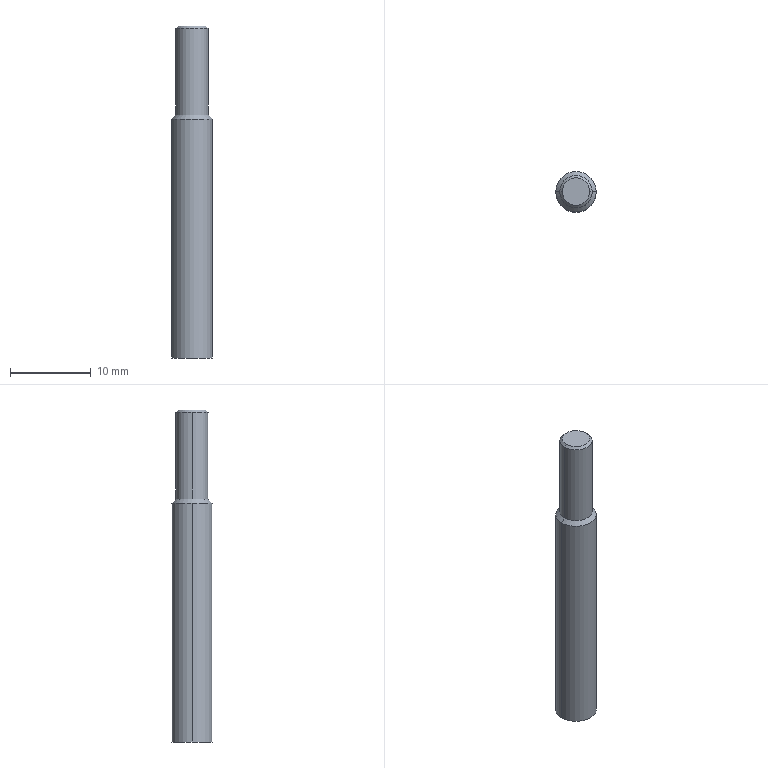Part | SolidWorks | features BaseBody 1 | 1 solid | 10 faces | box 5 x 5 x 41 mm | volume 724.909 mm3 | cylinder 4 | cone 4 | plane 2 | commonest cylinder face diameters 4 x2 5 x2
STEP:
#1=CARTESIAN_POINT('',(2.5,0.,0.));
#2=VERTEX_POINT('',#1);
#3=CARTESIAN_POINT('',(-2.5,0.,0.));
#4=VERTEX_POINT('',#3);
#5=CARTESIAN_POINT('',(0.,0.,0.));
#6=DIRECTION('',(0.,0.,1.));
#7=DIRECTION('',(1.,0.,0.));
#8=AXIS2_PLACEMENT_3D('',#5,#6,#7);
#9=CIRCLE('',#8,2.5);
#10=EDGE_CURVE('',#2,#4,#9,.T.);
#11=ORIENTED_EDGE('',*,*,#10,.T.);
#12=CARTESIAN_POINT('',(-2.5,0.,29.5));
#13=VERTEX_POINT('',#12);
#14=CARTESIAN_POINT('',(-2.5,0.,0.));
#15=DIRECTION('',(0.,0.,1.));
#16=VECTOR('',#15,1000.);
#17=LINE('',#14,#16);
#18=EDGE_CURVE('',#4,#13,#17,.T.);
#19=ORIENTED_EDGE('',*,*,#18,.T.);
#20=CARTESIAN_POINT('',(2.5,0.,29.5));
#21=VERTEX_POINT('',#20);
#22=CARTESIAN_POINT('',(0.,0.,29.5));
#23=DIRECTION('',(0.,0.,-1.));
#24=DIRECTION('',(1.,0.,0.));
#25=AXIS2_PLACEMENT_3D('',#22,#23,#24);
#26=CIRCLE('',#25,2.5);
#27=EDGE_CURVE('',#13,#21,#26,.T.);
#28=ORIENTED_EDGE('',*,*,#27,.T.);
#29=CARTESIAN_POINT('',(2.5,0.,0.));
#30=DIRECTION('',(0.,0.,1.));
#31=VECTOR('',#30,1000.);
#32=LINE('',#29,#31);
#33=EDGE_CURVE('',#2,#21,#32,.T.);
#34=ORIENTED_EDGE('',*,*,#33,.F.);
#35=EDGE_LOOP('',(#11,#19,#28,#34));
#36=FACE_OUTER_BOUND('',#35,.T.);
#37=CARTESIAN_POINT('',(0.,0.,0.));
#38=DIRECTION('',(0.,0.,1.));
#39=DIRECTION('',(1.,0.,0.));
#40=AXIS2_PLACEMENT_3D('',#37,#38,#39);
#41=CYLINDRICAL_SURFACE('',#40,2.5);
#42=ADVANCED_FACE('',(#36),#41,.T.);
#43=CARTESIAN_POINT('',(-2.,0.,30.));
#44=VERTEX_POINT('',#43);
#45=CARTESIAN_POINT('',(2.,0.,30.));
#46=VERTEX_POINT('',#45);
#47=CARTESIAN_POINT('',(0.,0.,30.));
#48=DIRECTION('',(0.,0.,-1.));
#49=DIRECTION('',(-1.,0.,0.));
#50=AXIS2_PLACEMENT_3D('',#47,#48,#49);
#51=CIRCLE('',#50,2.);
#52=EDGE_CURVE('',#44,#46,#51,.T.);
#53=ORIENTED_EDGE('',*,*,#52,.T.);
#54=CARTESIAN_POINT('',(2.5,0.,29.5));
#55=DIRECTION('',(0.7071,0.,-0.7071));
#56=VECTOR('',#55,1000.);
#57=LINE('',#54,#56);
#58=EDGE_CURVE('',#46,#21,#57,.T.);
#59=ORIENTED_EDGE('',*,*,#58,.T.);
#60=ORIENTED_EDGE('',*,*,#27,.F.);
#61=CARTESIAN_POINT('',(-2.5,0.,29.5));
#62=DIRECTION('',(-0.7071,0.,-0.7071));
#63=VECTOR('',#62,1000.);
#64=LINE('',#61,#63);
#65=EDGE_CURVE('',#44,#13,#64,.T.);
#66=ORIENTED_EDGE('',*,*,#65,.F.);
#67=EDGE_LOOP('',(#53,#59,#60,#66));
#68=FACE_OUTER_BOUND('',#67,.T.);
#69=CARTESIAN_POINT('',(0.,0.,29.5));
#70=DIRECTION('',(0.,0.,-1.));
#71=DIRECTION('',(-1.,0.,0.));
#72=AXIS2_PLACEMENT_3D('',#69,#70,#71);
#73=CONICAL_SURFACE('',#72,2.5,0.7854);
#74=ADVANCED_FACE('',(#68),#73,.T.);
#75=ORIENTED_EDGE('',*,*,#52,.F.);
#76=CARTESIAN_POINT('',(-2.,0.,40.7));
#77=VERTEX_POINT('',#76);
#78=CARTESIAN_POINT('',(-2.,0.,30.));
#79=DIRECTION('',(0.,0.,1.));
#80=VECTOR('',#79,1000.);
#81=LINE('',#78,#80);
#82=EDGE_CURVE('',#44,#77,#81,.T.);
#83=ORIENTED_EDGE('',*,*,#82,.T.);
#84=CARTESIAN_POINT('',(2.,0.,40.7));
#85=VERTEX_POINT('',#84);
#86=CARTESIAN_POINT('',(0.,0.,40.7));
#87=DIRECTION('',(0.,0.,-1.));
#88=DIRECTION('',(1.,0.,0.));
#89=AXIS2_PLACEMENT_3D('',#86,#87,#88);
#90=CIRCLE('',#89,2.);
#91=EDGE_CURVE('',#77,#85,#90,.T.);
#92=ORIENTED_EDGE('',*,*,#91,.T.);
#93=CARTESIAN_POINT('',(2.,0.,30.));
#94=DIRECTION('',(0.,0.,1.));
#95=VECTOR('',#94,1000.);
#96=LINE('',#93,#95);
#97=EDGE_CURVE('',#46,#85,#96,.T.);
#98=ORIENTED_EDGE('',*,*,#97,.F.);
#99=EDGE_LOOP('',(#75,#83,#92,#98));
#100=FACE_OUTER_BOUND('',#99,.T.);
#101=CARTESIAN_POINT('',(0.,0.,30.));
#102=DIRECTION('',(0.,0.,1.));
#103=DIRECTION('',(1.,0.,0.));
#104=AXIS2_PLACEMENT_3D('',#101,#102,#103);
#105=CYLINDRICAL_SURFACE('',#104,2.);
#106=ADVANCED_FACE('',(#100),#105,.T.);
#107=CARTESIAN_POINT('',(-1.7,0.,41.));
#108=VERTEX_POINT('',#107);
#109=CARTESIAN_POINT('',(1.7,0.,41.));
#110=VERTEX_POINT('',#109);
#111=CARTESIAN_POINT('',(0.,0.,41.));
#112=DIRECTION('',(0.,0.,-1.));
#113=DIRECTION('',(-1.,0.,0.));
#114=AXIS2_PLACEMENT_3D('',#111,#112,#113);
#115=CIRCLE('',#114,1.7);
#116=EDGE_CURVE('',#108,#110,#115,.T.);
#117=ORIENTED_EDGE('',*,*,#116,.T.);
#118=CARTESIAN_POINT('',(2.,0.,40.7));
#119=DIRECTION('',(0.7071,0.,-0.7071));
#120=VECTOR('',#119,1000.);
#121=LINE('',#118,#120);
#122=EDGE_CURVE('',#110,#85,#121,.T.);
#123=ORIENTED_EDGE('',*,*,#122,.T.);
#124=ORIENTED_EDGE('',*,*,#91,.F.);
#125=CARTESIAN_POINT('',(-2.,0.,40.7));
#126=DIRECTION('',(-0.7071,0.,-0.7071));
#127=VECTOR('',#126,1000.);
#128=LINE('',#125,#127);
#129=EDGE_CURVE('',#108,#77,#128,.T.);
#130=ORIENTED_EDGE('',*,*,#129,.F.);
#131=EDGE_LOOP('',(#117,#123,#124,#130));
#132=FACE_OUTER_BOUND('',#131,.T.);
#133=CARTESIAN_POINT('',(0.,0.,40.7));
#134=DIRECTION('',(0.,0.,-1.));
#135=DIRECTION('',(-1.,0.,0.));
#136=AXIS2_PLACEMENT_3D('',#133,#134,#135);
#137=CONICAL_SURFACE('',#136,2.,0.7854);
#138=ADVANCED_FACE('',(#132),#137,.T.);
#139=ORIENTED_EDGE('',*,*,#18,.F.);
#140=CARTESIAN_POINT('',(0.,0.,0.));
#141=DIRECTION('',(0.,0.,1.));
#142=DIRECTION('',(1.,0.,0.));
#143=AXIS2_PLACEMENT_3D('',#140,#141,#142);
#144=CIRCLE('',#143,2.5);
#145=EDGE_CURVE('',#4,#2,#144,.T.);
#146=ORIENTED_EDGE('',*,*,#145,.T.);
#147=ORIENTED_EDGE('',*,*,#33,.T.);
#148=CARTESIAN_POINT('',(0.,0.,29.5));
#149=DIRECTION('',(0.,0.,-1.));
#150=DIRECTION('',(1.,0.,0.));
#151=AXIS2_PLACEMENT_3D('',#148,#149,#150);
#152=CIRCLE('',#151,2.5);
#153=EDGE_CURVE('',#21,#13,#152,.T.);
#154=ORIENTED_EDGE('',*,*,#153,.T.);
#155=EDGE_LOOP('',(#139,#146,#147,#154));
#156=FACE_OUTER_BOUND('',#155,.T.);
#157=CARTESIAN_POINT('',(0.,0.,0.));
#158=DIRECTION('',(0.,0.,1.));
#159=DIRECTION('',(1.,0.,0.));
#160=AXIS2_PLACEMENT_3D('',#157,#158,#159);
#161=CYLINDRICAL_SURFACE('',#160,2.5);
#162=ADVANCED_FACE('',(#156),#161,.T.);
#163=ORIENTED_EDGE('',*,*,#58,.F.);
#164=CARTESIAN_POINT('',(0.,0.,30.));
#165=DIRECTION('',(0.,0.,-1.));
#166=DIRECTION('',(-1.,0.,0.));
#167=AXIS2_PLACEMENT_3D('',#164,#165,#166);
#168=CIRCLE('',#167,2.);
#169=EDGE_CURVE('',#46,#44,#168,.T.);
#170=ORIENTED_EDGE('',*,*,#169,.T.);
#171=ORIENTED_EDGE('',*,*,#65,.T.);
#172=ORIENTED_EDGE('',*,*,#153,.F.);
#173=EDGE_LOOP('',(#163,#170,#171,#172));
#174=FACE_OUTER_BOUND('',#173,.T.);
#175=CARTESIAN_POINT('',(0.,0.,29.5));
#176=DIRECTION('',(0.,0.,-1.));
#177=DIRECTION('',(-1.,0.,0.));
#178=AXIS2_PLACEMENT_3D('',#175,#176,#177);
#179=CONICAL_SURFACE('',#178,2.5,0.7854);
#180=ADVANCED_FACE('',(#174),#179,.T.);
#181=ORIENTED_EDGE('',*,*,#10,.F.);
#182=ORIENTED_EDGE('',*,*,#145,.F.);
#183=EDGE_LOOP('',(#181,#182));
#184=FACE_OUTER_BOUND('',#183,.T.);
#185=CARTESIAN_POINT('',(0.,0.,0.));
#186=DIRECTION('',(0.,0.,-1.));
#187=DIRECTION('',(-1.,0.,0.));
#188=AXIS2_PLACEMENT_3D('',#185,#186,#187);
#189=PLANE('',#188);
#190=ADVANCED_FACE('',(#184),#189,.T.);
#191=ORIENTED_EDGE('',*,*,#82,.F.);
#192=ORIENTED_EDGE('',*,*,#169,.F.);
#193=ORIENTED_EDGE('',*,*,#97,.T.);
#194=CARTESIAN_POINT('',(0.,0.,40.7));
#195=DIRECTION('',(0.,0.,-1.));
#196=DIRECTION('',(1.,0.,0.));
#197=AXIS2_PLACEMENT_3D('',#194,#195,#196);
#198=CIRCLE('',#197,2.);
#199=EDGE_CURVE('',#85,#77,#198,.T.);
#200=ORIENTED_EDGE('',*,*,#199,.T.);
#201=EDGE_LOOP('',(#191,#192,#193,#200));
#202=FACE_OUTER_BOUND('',#201,.T.);
#203=CARTESIAN_POINT('',(0.,0.,30.));
#204=DIRECTION('',(0.,0.,1.));
#205=DIRECTION('',(1.,0.,0.));
#206=AXIS2_PLACEMENT_3D('',#203,#204,#205);
#207=CYLINDRICAL_SURFACE('',#206,2.);
#208=ADVANCED_FACE('',(#202),#207,.T.);
#209=ORIENTED_EDGE('',*,*,#122,.F.);
#210=CARTESIAN_POINT('',(0.,0.,41.));
#211=DIRECTION('',(0.,0.,-1.));
#212=DIRECTION('',(-1.,0.,0.));
#213=AXIS2_PLACEMENT_3D('',#210,#211,#212);
#214=CIRCLE('',#213,1.7);
#215=EDGE_CURVE('',#110,#108,#214,.T.);
#216=ORIENTED_EDGE('',*,*,#215,.T.);
#217=ORIENTED_EDGE('',*,*,#129,.T.);
#218=ORIENTED_EDGE('',*,*,#199,.F.);
#219=EDGE_LOOP('',(#209,#216,#217,#218));
#220=FACE_OUTER_BOUND('',#219,.T.);
#221=CARTESIAN_POINT('',(0.,0.,40.7));
#222=DIRECTION('',(0.,0.,-1.));
#223=DIRECTION('',(-1.,0.,0.));
#224=AXIS2_PLACEMENT_3D('',#221,#222,#223);
#225=CONICAL_SURFACE('',#224,2.,0.7854);
#226=ADVANCED_FACE('',(#220),#225,.T.);
#227=ORIENTED_EDGE('',*,*,#116,.F.);
#228=ORIENTED_EDGE('',*,*,#215,.F.);
#229=EDGE_LOOP('',(#227,#228));
#230=FACE_OUTER_BOUND('',#229,.T.);
#231=CARTESIAN_POINT('',(0.,0.,41.));
#232=DIRECTION('',(0.,0.,-1.));
#233=DIRECTION('',(-1.,0.,0.));
#234=AXIS2_PLACEMENT_3D('',#231,#232,#233);
#235=PLANE('',#234);
#236=ADVANCED_FACE('',(#230),#235,.F.);
#237=CLOSED_SHELL('',(#42,#74,#106,#138,#162,#180,#190,#208,#226,#236));
#238=MANIFOLD_SOLID_BREP('',#237);
#239=CARTESIAN_POINT('',(0.,0.,0.));
#240=DIRECTION('',(0.,0.,1.));
#241=DIRECTION('',(1.,0.,0.));
#242=AXIS2_PLACEMENT_3D('',#239,#240,#241);
#243=(LENGTH_UNIT()NAMED_UNIT(*)SI_UNIT(.MILLI.,.METRE.));
#244=UNCERTAINTY_MEASURE_WITH_UNIT(LENGTH_MEASURE(0.00001),#243,'','');
#245=(NAMED_UNIT(*)PLANE_ANGLE_UNIT()SI_UNIT($,.RADIAN.));
#246=(NAMED_UNIT(*)SI_UNIT($,.STERADIAN.)SOLID_ANGLE_UNIT());
#247=(GEOMETRIC_REPRESENTATION_CONTEXT(3)GLOBAL_UNCERTAINTY_ASSIGNED_CONTEXT((#244))GLOBAL_UNIT_ASSIGNED_CONTEXT((#243,#245,#246))REPRESENTATION_CONTEXT('',''));
#248=ADVANCED_BREP_SHAPE_REPRESENTATION('',(#238,#242),#247);